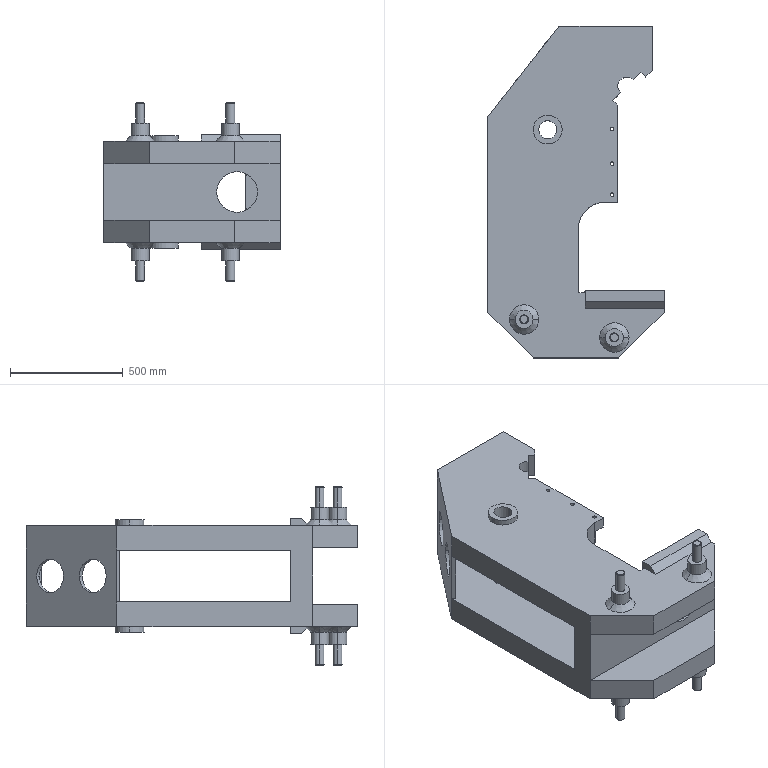Part | Creo | features CURVE 13, PROTRUSION 10, CUT 7, CHAMFER 3, DATUM PLANE 3, MIRROR 3, COORDINATE SYSTEM 1 | 1 solid | 146 faces | box 780 x 1470 x 790 mm | volume 186494626 mm3 | plane 70 | cylinder 60 | cone 16 | commonest cylinder face diameters 40 x16 80 x16 16 x12 128 x4 150 x4 60 x2